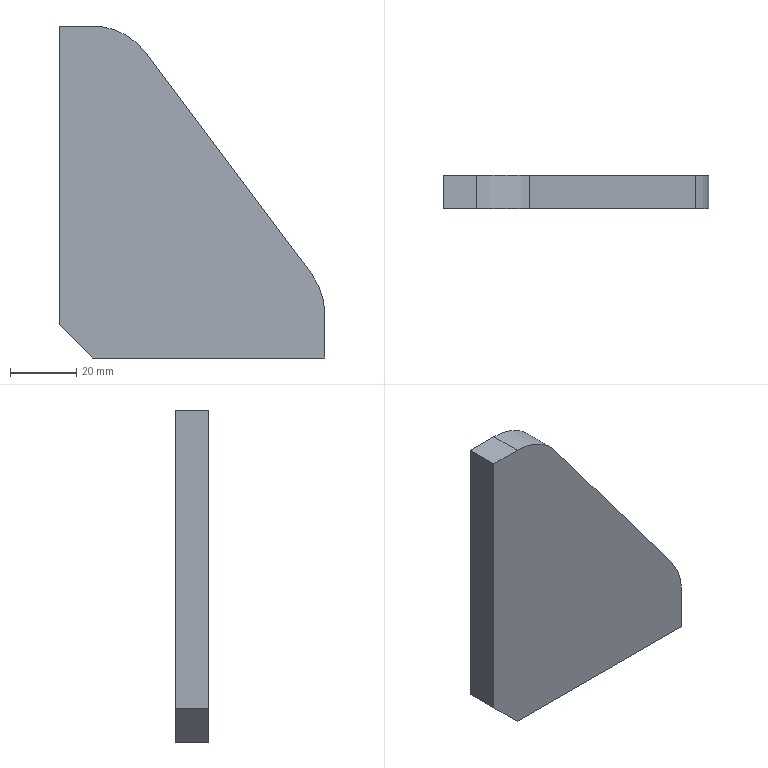Part | SolidWorks | features BaseBody 1 | 1 solid | 10 faces | box 80 x 10 x 100 mm | volume 55308 mm3 | plane 8 | cylinder 2 | commonest cylinder face diameters 40 x2
STEP:
#1=CARTESIAN_POINT('',(40.,-5.,-50.));
#2=VERTEX_POINT('',#1);
#3=CARTESIAN_POINT('',(-30.,-5.,-50.));
#4=VERTEX_POINT('',#3);
#5=CARTESIAN_POINT('',(40.,-5.,-50.));
#6=DIRECTION('',(-1.,0.,0.));
#7=VECTOR('',#6,1000.);
#8=LINE('',#5,#7);
#9=EDGE_CURVE('',#2,#4,#8,.T.);
#10=ORIENTED_EDGE('',*,*,#9,.T.);
#11=CARTESIAN_POINT('',(-30.,5.,-50.));
#12=VERTEX_POINT('',#11);
#13=CARTESIAN_POINT('',(-30.,5.,-50.));
#14=DIRECTION('',(0.,-1.,0.));
#15=VECTOR('',#14,1000.);
#16=LINE('',#13,#15);
#17=EDGE_CURVE('',#12,#4,#16,.T.);
#18=ORIENTED_EDGE('',*,*,#17,.F.);
#19=CARTESIAN_POINT('',(40.,5.,-50.));
#20=VERTEX_POINT('',#19);
#21=CARTESIAN_POINT('',(40.,5.,-50.));
#22=DIRECTION('',(-1.,0.,0.));
#23=VECTOR('',#22,1000.);
#24=LINE('',#21,#23);
#25=EDGE_CURVE('',#20,#12,#24,.T.);
#26=ORIENTED_EDGE('',*,*,#25,.F.);
#27=CARTESIAN_POINT('',(40.,5.,-50.));
#28=DIRECTION('',(0.,-1.,0.));
#29=VECTOR('',#28,1000.);
#30=LINE('',#27,#29);
#31=EDGE_CURVE('',#20,#2,#30,.T.);
#32=ORIENTED_EDGE('',*,*,#31,.T.);
#33=EDGE_LOOP('',(#10,#18,#26,#32));
#34=FACE_OUTER_BOUND('',#33,.T.);
#35=CARTESIAN_POINT('',(40.,5.,-50.));
#36=DIRECTION('',(0.,0.,1.));
#37=DIRECTION('',(1.,0.,0.));
#38=AXIS2_PLACEMENT_3D('',#35,#36,#37);
#39=PLANE('',#38);
#40=ADVANCED_FACE('',(#34),#39,.F.);
#41=CARTESIAN_POINT('',(-40.,-5.,-40.));
#42=VERTEX_POINT('',#41);
#43=CARTESIAN_POINT('',(-30.,-5.,-50.));
#44=DIRECTION('',(-0.7071,0.,0.7071));
#45=VECTOR('',#44,1000.);
#46=LINE('',#43,#45);
#47=EDGE_CURVE('',#4,#42,#46,.T.);
#48=ORIENTED_EDGE('',*,*,#47,.T.);
#49=CARTESIAN_POINT('',(-40.,5.,-40.));
#50=VERTEX_POINT('',#49);
#51=CARTESIAN_POINT('',(-40.,5.,-40.));
#52=DIRECTION('',(0.,-1.,0.));
#53=VECTOR('',#52,1000.);
#54=LINE('',#51,#53);
#55=EDGE_CURVE('',#50,#42,#54,.T.);
#56=ORIENTED_EDGE('',*,*,#55,.F.);
#57=CARTESIAN_POINT('',(-30.,5.,-50.));
#58=DIRECTION('',(-0.7071,0.,0.7071));
#59=VECTOR('',#58,1000.);
#60=LINE('',#57,#59);
#61=EDGE_CURVE('',#12,#50,#60,.T.);
#62=ORIENTED_EDGE('',*,*,#61,.F.);
#63=ORIENTED_EDGE('',*,*,#17,.T.);
#64=EDGE_LOOP('',(#48,#56,#62,#63));
#65=FACE_OUTER_BOUND('',#64,.T.);
#66=CARTESIAN_POINT('',(-30.,5.,-50.));
#67=DIRECTION('',(0.7071,0.,0.7071));
#68=DIRECTION('',(0.7071,0.,-0.7071));
#69=AXIS2_PLACEMENT_3D('',#66,#67,#68);
#70=PLANE('',#69);
#71=ADVANCED_FACE('',(#65),#70,.F.);
#72=CARTESIAN_POINT('',(-40.,-5.,50.));
#73=VERTEX_POINT('',#72);
#74=CARTESIAN_POINT('',(-40.,-5.,-40.));
#75=DIRECTION('',(0.,0.,1.));
#76=VECTOR('',#75,1000.);
#77=LINE('',#74,#76);
#78=EDGE_CURVE('',#42,#73,#77,.T.);
#79=ORIENTED_EDGE('',*,*,#78,.T.);
#80=CARTESIAN_POINT('',(-40.,5.,50.));
#81=VERTEX_POINT('',#80);
#82=CARTESIAN_POINT('',(-40.,5.,50.));
#83=DIRECTION('',(0.,-1.,0.));
#84=VECTOR('',#83,1000.);
#85=LINE('',#82,#84);
#86=EDGE_CURVE('',#81,#73,#85,.T.);
#87=ORIENTED_EDGE('',*,*,#86,.F.);
#88=CARTESIAN_POINT('',(-40.,5.,-40.));
#89=DIRECTION('',(0.,0.,1.));
#90=VECTOR('',#89,1000.);
#91=LINE('',#88,#90);
#92=EDGE_CURVE('',#50,#81,#91,.T.);
#93=ORIENTED_EDGE('',*,*,#92,.F.);
#94=ORIENTED_EDGE('',*,*,#55,.T.);
#95=EDGE_LOOP('',(#79,#87,#93,#94));
#96=FACE_OUTER_BOUND('',#95,.T.);
#97=CARTESIAN_POINT('',(-40.,5.,-40.));
#98=DIRECTION('',(1.,0.,0.));
#99=DIRECTION('',(0.,0.,-1.));
#100=AXIS2_PLACEMENT_3D('',#97,#98,#99);
#101=PLANE('',#100);
#102=ADVANCED_FACE('',(#96),#101,.F.);
#103=CARTESIAN_POINT('',(-30.,-5.,50.));
#104=VERTEX_POINT('',#103);
#105=CARTESIAN_POINT('',(-40.,-5.,50.));
#106=DIRECTION('',(1.,0.,0.));
#107=VECTOR('',#106,1000.);
#108=LINE('',#105,#107);
#109=EDGE_CURVE('',#73,#104,#108,.T.);
#110=ORIENTED_EDGE('',*,*,#109,.T.);
#111=CARTESIAN_POINT('',(-30.,5.,50.));
#112=VERTEX_POINT('',#111);
#113=CARTESIAN_POINT('',(-30.,5.,50.));
#114=DIRECTION('',(0.,-1.,0.));
#115=VECTOR('',#114,1000.);
#116=LINE('',#113,#115);
#117=EDGE_CURVE('',#112,#104,#116,.T.);
#118=ORIENTED_EDGE('',*,*,#117,.F.);
#119=CARTESIAN_POINT('',(-40.,5.,50.));
#120=DIRECTION('',(1.,0.,0.));
#121=VECTOR('',#120,1000.);
#122=LINE('',#119,#121);
#123=EDGE_CURVE('',#81,#112,#122,.T.);
#124=ORIENTED_EDGE('',*,*,#123,.F.);
#125=ORIENTED_EDGE('',*,*,#86,.T.);
#126=EDGE_LOOP('',(#110,#118,#124,#125));
#127=FACE_OUTER_BOUND('',#126,.T.);
#128=CARTESIAN_POINT('',(-40.,5.,50.));
#129=DIRECTION('',(0.,0.,-1.));
#130=DIRECTION('',(-1.,0.,0.));
#131=AXIS2_PLACEMENT_3D('',#128,#129,#130);
#132=PLANE('',#131);
#133=ADVANCED_FACE('',(#127),#132,.F.);
#134=CARTESIAN_POINT('',(-14.,-5.,42.));
#135=VERTEX_POINT('',#134);
#136=CARTESIAN_POINT('',(-30.,-5.,30.));
#137=DIRECTION('',(0.,1.,0.));
#138=DIRECTION('',(0.,0.,1.));
#139=AXIS2_PLACEMENT_3D('',#136,#137,#138);
#140=CIRCLE('',#139,20.);
#141=EDGE_CURVE('',#104,#135,#140,.T.);
#142=ORIENTED_EDGE('',*,*,#141,.T.);
#143=CARTESIAN_POINT('',(-14.,5.,42.));
#144=VERTEX_POINT('',#143);
#145=CARTESIAN_POINT('',(-14.,5.,42.));
#146=DIRECTION('',(0.,-1.,0.));
#147=VECTOR('',#146,1000.);
#148=LINE('',#145,#147);
#149=EDGE_CURVE('',#144,#135,#148,.T.);
#150=ORIENTED_EDGE('',*,*,#149,.F.);
#151=CARTESIAN_POINT('',(-30.,5.,30.));
#152=DIRECTION('',(0.,1.,0.));
#153=DIRECTION('',(0.,0.,1.));
#154=AXIS2_PLACEMENT_3D('',#151,#152,#153);
#155=CIRCLE('',#154,20.);
#156=EDGE_CURVE('',#112,#144,#155,.T.);
#157=ORIENTED_EDGE('',*,*,#156,.F.);
#158=ORIENTED_EDGE('',*,*,#117,.T.);
#159=EDGE_LOOP('',(#142,#150,#157,#158));
#160=FACE_OUTER_BOUND('',#159,.T.);
#161=CARTESIAN_POINT('',(-30.,5.,30.));
#162=DIRECTION('',(0.,-1.,0.));
#163=DIRECTION('',(0.,0.,-1.));
#164=AXIS2_PLACEMENT_3D('',#161,#162,#163);
#165=CYLINDRICAL_SURFACE('',#164,20.);
#166=ADVANCED_FACE('',(#160),#165,.T.);
#167=CARTESIAN_POINT('',(36.,-5.,-24.667));
#168=VERTEX_POINT('',#167);
#169=CARTESIAN_POINT('',(-14.,-5.,42.));
#170=DIRECTION('',(0.6,0.,-0.8));
#171=VECTOR('',#170,1000.);
#172=LINE('',#169,#171);
#173=EDGE_CURVE('',#135,#168,#172,.T.);
#174=ORIENTED_EDGE('',*,*,#173,.T.);
#175=CARTESIAN_POINT('',(36.,5.,-24.667));
#176=VERTEX_POINT('',#175);
#177=CARTESIAN_POINT('',(36.,5.,-24.667));
#178=DIRECTION('',(0.,-1.,0.));
#179=VECTOR('',#178,1000.);
#180=LINE('',#177,#179);
#181=EDGE_CURVE('',#176,#168,#180,.T.);
#182=ORIENTED_EDGE('',*,*,#181,.F.);
#183=CARTESIAN_POINT('',(-14.,5.,42.));
#184=DIRECTION('',(0.6,0.,-0.8));
#185=VECTOR('',#184,1000.);
#186=LINE('',#183,#185);
#187=EDGE_CURVE('',#144,#176,#186,.T.);
#188=ORIENTED_EDGE('',*,*,#187,.F.);
#189=ORIENTED_EDGE('',*,*,#149,.T.);
#190=EDGE_LOOP('',(#174,#182,#188,#189));
#191=FACE_OUTER_BOUND('',#190,.T.);
#192=CARTESIAN_POINT('',(-14.,5.,42.));
#193=DIRECTION('',(-0.8,0.,-0.6));
#194=DIRECTION('',(-0.6,0.,0.8));
#195=AXIS2_PLACEMENT_3D('',#192,#193,#194);
#196=PLANE('',#195);
#197=ADVANCED_FACE('',(#191),#196,.F.);
#198=CARTESIAN_POINT('',(40.,-5.,-36.667));
#199=VERTEX_POINT('',#198);
#200=CARTESIAN_POINT('',(20.,-5.,-36.667));
#201=DIRECTION('',(0.,1.,0.));
#202=DIRECTION('',(0.,0.,-1.));
#203=AXIS2_PLACEMENT_3D('',#200,#201,#202);
#204=CIRCLE('',#203,20.);
#205=EDGE_CURVE('',#168,#199,#204,.T.);
#206=ORIENTED_EDGE('',*,*,#205,.T.);
#207=CARTESIAN_POINT('',(40.,5.,-36.667));
#208=VERTEX_POINT('',#207);
#209=CARTESIAN_POINT('',(40.,5.,-36.667));
#210=DIRECTION('',(0.,-1.,0.));
#211=VECTOR('',#210,1000.);
#212=LINE('',#209,#211);
#213=EDGE_CURVE('',#208,#199,#212,.T.);
#214=ORIENTED_EDGE('',*,*,#213,.F.);
#215=CARTESIAN_POINT('',(20.,5.,-36.667));
#216=DIRECTION('',(0.,1.,0.));
#217=DIRECTION('',(0.,0.,-1.));
#218=AXIS2_PLACEMENT_3D('',#215,#216,#217);
#219=CIRCLE('',#218,20.);
#220=EDGE_CURVE('',#176,#208,#219,.T.);
#221=ORIENTED_EDGE('',*,*,#220,.F.);
#222=ORIENTED_EDGE('',*,*,#181,.T.);
#223=EDGE_LOOP('',(#206,#214,#221,#222));
#224=FACE_OUTER_BOUND('',#223,.T.);
#225=CARTESIAN_POINT('',(20.,5.,-36.667));
#226=DIRECTION('',(0.,-1.,0.));
#227=DIRECTION('',(0.,0.,-1.));
#228=AXIS2_PLACEMENT_3D('',#225,#226,#227);
#229=CYLINDRICAL_SURFACE('',#228,20.);
#230=ADVANCED_FACE('',(#224),#229,.T.);
#231=CARTESIAN_POINT('',(40.,-5.,-36.667));
#232=DIRECTION('',(0.,0.,-1.));
#233=VECTOR('',#232,1000.);
#234=LINE('',#231,#233);
#235=EDGE_CURVE('',#199,#2,#234,.T.);
#236=ORIENTED_EDGE('',*,*,#235,.T.);
#237=ORIENTED_EDGE('',*,*,#31,.F.);
#238=CARTESIAN_POINT('',(40.,5.,-36.667));
#239=DIRECTION('',(0.,0.,-1.));
#240=VECTOR('',#239,1000.);
#241=LINE('',#238,#240);
#242=EDGE_CURVE('',#208,#20,#241,.T.);
#243=ORIENTED_EDGE('',*,*,#242,.F.);
#244=ORIENTED_EDGE('',*,*,#213,.T.);
#245=EDGE_LOOP('',(#236,#237,#243,#244));
#246=FACE_OUTER_BOUND('',#245,.T.);
#247=CARTESIAN_POINT('',(40.,5.,-36.667));
#248=DIRECTION('',(-1.,0.,0.));
#249=DIRECTION('',(0.,0.,1.));
#250=AXIS2_PLACEMENT_3D('',#247,#248,#249);
#251=PLANE('',#250);
#252=ADVANCED_FACE('',(#246),#251,.F.);
#253=ORIENTED_EDGE('',*,*,#25,.T.);
#254=ORIENTED_EDGE('',*,*,#61,.T.);
#255=ORIENTED_EDGE('',*,*,#92,.T.);
#256=ORIENTED_EDGE('',*,*,#123,.T.);
#257=ORIENTED_EDGE('',*,*,#156,.T.);
#258=ORIENTED_EDGE('',*,*,#187,.T.);
#259=ORIENTED_EDGE('',*,*,#220,.T.);
#260=ORIENTED_EDGE('',*,*,#242,.T.);
#261=EDGE_LOOP('',(#253,#254,#255,#256,#257,#258,#259,#260));
#262=FACE_OUTER_BOUND('',#261,.T.);
#263=CARTESIAN_POINT('',(-30.,5.,30.));
#264=DIRECTION('',(0.,1.,0.));
#265=DIRECTION('',(0.,0.,1.));
#266=AXIS2_PLACEMENT_3D('',#263,#264,#265);
#267=PLANE('',#266);
#268=ADVANCED_FACE('',(#262),#267,.T.);
#269=ORIENTED_EDGE('',*,*,#9,.F.);
#270=ORIENTED_EDGE('',*,*,#235,.F.);
#271=ORIENTED_EDGE('',*,*,#205,.F.);
#272=ORIENTED_EDGE('',*,*,#173,.F.);
#273=ORIENTED_EDGE('',*,*,#141,.F.);
#274=ORIENTED_EDGE('',*,*,#109,.F.);
#275=ORIENTED_EDGE('',*,*,#78,.F.);
#276=ORIENTED_EDGE('',*,*,#47,.F.);
#277=EDGE_LOOP('',(#269,#270,#271,#272,#273,#274,#275,#276));
#278=FACE_OUTER_BOUND('',#277,.T.);
#279=CARTESIAN_POINT('',(-30.,-5.,30.));
#280=DIRECTION('',(0.,1.,0.));
#281=DIRECTION('',(0.,0.,1.));
#282=AXIS2_PLACEMENT_3D('',#279,#280,#281);
#283=PLANE('',#282);
#284=ADVANCED_FACE('',(#278),#283,.F.);
#285=CLOSED_SHELL('',(#40,#71,#102,#133,#166,#197,#230,#252,#268,#284));
#286=MANIFOLD_SOLID_BREP('',#285);
#287=CARTESIAN_POINT('',(0.,0.,0.));
#288=DIRECTION('',(0.,0.,1.));
#289=DIRECTION('',(1.,0.,0.));
#290=AXIS2_PLACEMENT_3D('',#287,#288,#289);
#291=(LENGTH_UNIT()NAMED_UNIT(*)SI_UNIT(.MILLI.,.METRE.));
#292=UNCERTAINTY_MEASURE_WITH_UNIT(LENGTH_MEASURE(0.00001),#291,'','');
#293=(NAMED_UNIT(*)PLANE_ANGLE_UNIT()SI_UNIT($,.RADIAN.));
#294=(NAMED_UNIT(*)SI_UNIT($,.STERADIAN.)SOLID_ANGLE_UNIT());
#295=(GEOMETRIC_REPRESENTATION_CONTEXT(3)GLOBAL_UNCERTAINTY_ASSIGNED_CONTEXT((#292))GLOBAL_UNIT_ASSIGNED_CONTEXT((#291,#293,#294))REPRESENTATION_CONTEXT('',''));
#296=ADVANCED_BREP_SHAPE_REPRESENTATION('',(#286,#290),#295);